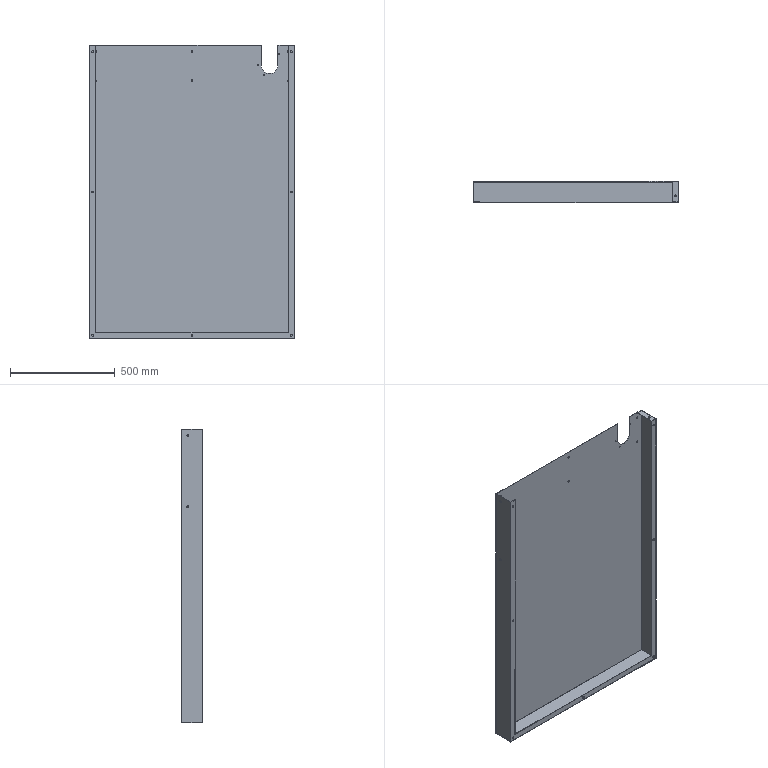Part | SolidWorks | features ICE 8, Extrusion 1, HoleWzd 1, Shell 1 | 1 solid | 57 faces | box 980 x 100 x 1400 mm | volume 3675222 mm3 | cylinder 39 | plane 18 | commonest cylinder face diameters 9 x32 4.2 x6 80.006 x1